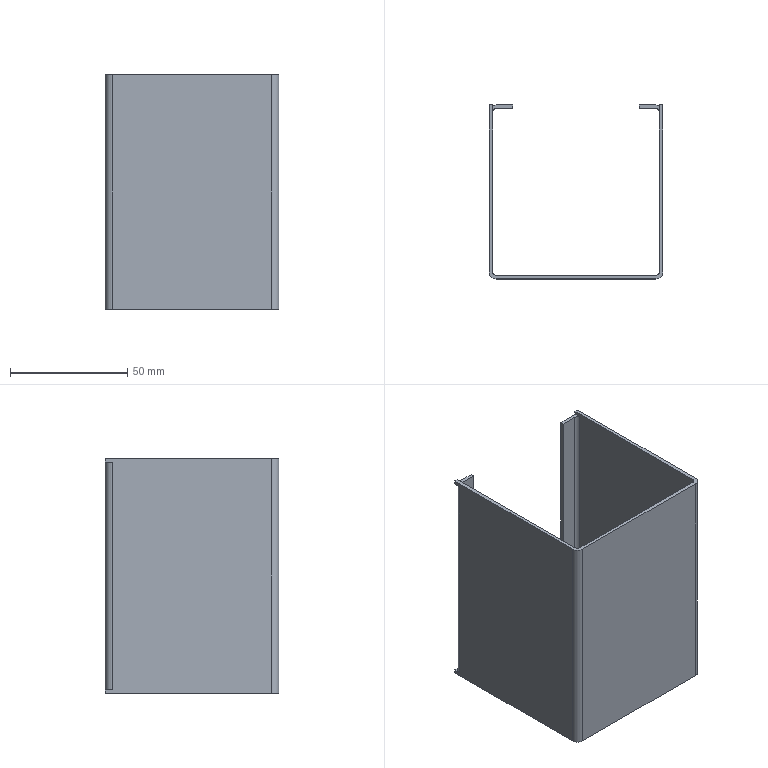Part | NX | features solid 2 | 1 solid | 38 faces | box 74 x 74 x 100 mm | volume 34746 mm3 | plane 30 | cylinder 8 | commonest cylinder face diameters 3 x4 6 x4
STEP:
#1=CARTESIAN_POINT('',(-974.5,-1370.,1296.6));
#2=VERTEX_POINT('',#1);
#3=CARTESIAN_POINT('',(-974.5,-1370.,1393.4));
#4=VERTEX_POINT('',#3);
#5=CARTESIAN_POINT('',(-974.5,-1370.,1296.6));
#6=DIRECTION('',(0.,0.,1.));
#7=VECTOR('',#6,1000.);
#8=LINE('',#5,#7);
#9=EDGE_CURVE('',#2,#4,#8,.T.);
#10=ORIENTED_EDGE('',*,*,#9,.T.);
#11=CARTESIAN_POINT('',(-976.,-1368.5,1393.4));
#12=VERTEX_POINT('',#11);
#13=CARTESIAN_POINT('',(-976.,-1370.,1393.4));
#14=DIRECTION('',(0.,0.,-1.));
#15=DIRECTION('',(1.,0.,0.));
#16=AXIS2_PLACEMENT_3D('',#13,#14,#15);
#17=CIRCLE('',#16,1.5);
#18=EDGE_CURVE('',#12,#4,#17,.T.);
#19=ORIENTED_EDGE('',*,*,#18,.F.);
#20=CARTESIAN_POINT('',(-976.,-1368.5,1296.6));
#21=VERTEX_POINT('',#20);
#22=CARTESIAN_POINT('',(-976.,-1368.5,1393.4));
#23=DIRECTION('',(0.,0.,-1.));
#24=VECTOR('',#23,1000.);
#25=LINE('',#22,#24);
#26=EDGE_CURVE('',#12,#21,#25,.T.);
#27=ORIENTED_EDGE('',*,*,#26,.T.);
#28=CARTESIAN_POINT('',(-976.,-1370.,1296.6));
#29=DIRECTION('',(0.,0.,-1.));
#30=DIRECTION('',(1.,0.,0.));
#31=AXIS2_PLACEMENT_3D('',#28,#29,#30);
#32=CIRCLE('',#31,1.5);
#33=EDGE_CURVE('',#21,#2,#32,.T.);
#34=ORIENTED_EDGE('',*,*,#33,.T.);
#35=EDGE_LOOP('',(#10,#19,#27,#34));
#36=FACE_BOUND('',#35,.T.);
#37=CARTESIAN_POINT('',(-976.,-1370.,1296.6));
#38=DIRECTION('',(0.,0.,1.));
#39=DIRECTION('',(-1.,0.,0.));
#40=AXIS2_PLACEMENT_3D('',#37,#38,#39);
#41=CYLINDRICAL_SURFACE('',#40,1.5);
#42=ADVANCED_FACE('',(#36),#41,.F.);
#43=CARTESIAN_POINT('',(-973.,-1370.,1296.6));
#44=VERTEX_POINT('',#43);
#45=CARTESIAN_POINT('',(-973.,-1370.,1393.4));
#46=VERTEX_POINT('',#45);
#47=CARTESIAN_POINT('',(-973.,-1370.,1296.6));
#48=DIRECTION('',(0.,0.,1.));
#49=VECTOR('',#48,1000.);
#50=LINE('',#47,#49);
#51=EDGE_CURVE('',#44,#46,#50,.T.);
#52=ORIENTED_EDGE('',*,*,#51,.F.);
#53=CARTESIAN_POINT('',(-976.,-1367.,1296.6));
#54=VERTEX_POINT('',#53);
#55=CARTESIAN_POINT('',(-976.,-1370.,1296.6));
#56=DIRECTION('',(0.,0.,-1.));
#57=DIRECTION('',(-1.,0.,0.));
#58=AXIS2_PLACEMENT_3D('',#55,#56,#57);
#59=CIRCLE('',#58,3.);
#60=EDGE_CURVE('',#54,#44,#59,.T.);
#61=ORIENTED_EDGE('',*,*,#60,.F.);
#62=CARTESIAN_POINT('',(-976.,-1367.,1393.4));
#63=VERTEX_POINT('',#62);
#64=CARTESIAN_POINT('',(-976.,-1367.,1393.4));
#65=DIRECTION('',(0.,0.,-1.));
#66=VECTOR('',#65,1000.);
#67=LINE('',#64,#66);
#68=EDGE_CURVE('',#63,#54,#67,.T.);
#69=ORIENTED_EDGE('',*,*,#68,.F.);
#70=CARTESIAN_POINT('',(-976.,-1370.,1393.4));
#71=DIRECTION('',(0.,0.,-1.));
#72=DIRECTION('',(-1.,0.,0.));
#73=AXIS2_PLACEMENT_3D('',#70,#71,#72);
#74=CIRCLE('',#73,3.);
#75=EDGE_CURVE('',#63,#46,#74,.T.);
#76=ORIENTED_EDGE('',*,*,#75,.T.);
#77=EDGE_LOOP('',(#52,#61,#69,#76));
#78=FACE_BOUND('',#77,.T.);
#79=CARTESIAN_POINT('',(-976.,-1370.,1296.6));
#80=DIRECTION('',(0.,0.,1.));
#81=DIRECTION('',(-1.,0.,0.));
#82=AXIS2_PLACEMENT_3D('',#79,#80,#81);
#83=CYLINDRICAL_SURFACE('',#82,3.);
#84=ADVANCED_FACE('',(#78),#83,.T.);
#85=CARTESIAN_POINT('',(-983.,-1368.5,1296.6));
#86=VERTEX_POINT('',#85);
#87=CARTESIAN_POINT('',(-983.,-1368.5,1393.4));
#88=VERTEX_POINT('',#87);
#89=CARTESIAN_POINT('',(-983.,-1368.5,1296.6));
#90=DIRECTION('',(0.,0.,1.));
#91=VECTOR('',#90,1000.);
#92=LINE('',#89,#91);
#93=EDGE_CURVE('',#86,#88,#92,.T.);
#94=ORIENTED_EDGE('',*,*,#93,.T.);
#95=CARTESIAN_POINT('',(-983.,-1367.,1393.4));
#96=VERTEX_POINT('',#95);
#97=CARTESIAN_POINT('',(-983.,-1367.,1393.4));
#98=DIRECTION('',(0.,-1.,0.));
#99=VECTOR('',#98,1000.);
#100=LINE('',#97,#99);
#101=EDGE_CURVE('',#96,#88,#100,.T.);
#102=ORIENTED_EDGE('',*,*,#101,.F.);
#103=CARTESIAN_POINT('',(-983.,-1367.,1296.6));
#104=VERTEX_POINT('',#103);
#105=CARTESIAN_POINT('',(-983.,-1367.,1296.6));
#106=DIRECTION('',(0.,0.,1.));
#107=VECTOR('',#106,1000.);
#108=LINE('',#105,#107);
#109=EDGE_CURVE('',#104,#96,#108,.T.);
#110=ORIENTED_EDGE('',*,*,#109,.F.);
#111=CARTESIAN_POINT('',(-983.,-1367.,1296.6));
#112=DIRECTION('',(0.,-1.,0.));
#113=VECTOR('',#112,1000.);
#114=LINE('',#111,#113);
#115=EDGE_CURVE('',#104,#86,#114,.T.);
#116=ORIENTED_EDGE('',*,*,#115,.T.);
#117=EDGE_LOOP('',(#94,#102,#110,#116));
#118=FACE_BOUND('',#117,.T.);
#119=CARTESIAN_POINT('',(-983.,-1367.,1296.6));
#120=DIRECTION('',(1.,0.,0.));
#121=DIRECTION('',(0.,0.,1.));
#122=AXIS2_PLACEMENT_3D('',#119,#120,#121);
#123=PLANE('',#122);
#124=ADVANCED_FACE('',(#118),#123,.F.);
#125=ORIENTED_EDGE('',*,*,#26,.F.);
#126=CARTESIAN_POINT('',(-983.,-1368.5,1393.4));
#127=DIRECTION('',(1.,0.,0.));
#128=VECTOR('',#127,1000.);
#129=LINE('',#126,#128);
#130=EDGE_CURVE('',#88,#12,#129,.T.);
#131=ORIENTED_EDGE('',*,*,#130,.F.);
#132=ORIENTED_EDGE('',*,*,#93,.F.);
#133=CARTESIAN_POINT('',(-974.351,-1368.5,1296.6));
#134=DIRECTION('',(-1.,0.,0.));
#135=VECTOR('',#134,1000.);
#136=LINE('',#133,#135);
#137=EDGE_CURVE('',#21,#86,#136,.T.);
#138=ORIENTED_EDGE('',*,*,#137,.F.);
#139=EDGE_LOOP('',(#125,#131,#132,#138));
#140=FACE_BOUND('',#139,.T.);
#141=CARTESIAN_POINT('',(-1010.,-1368.5,1345.));
#142=DIRECTION('',(0.,1.,0.));
#143=DIRECTION('',(1.,0.,0.));
#144=AXIS2_PLACEMENT_3D('',#141,#142,#143);
#145=PLANE('',#144);
#146=ADVANCED_FACE('',(#140),#145,.F.);
#147=CARTESIAN_POINT('',(-983.,-1367.,1393.4));
#148=DIRECTION('',(1.,0.,0.));
#149=VECTOR('',#148,1000.);
#150=LINE('',#147,#149);
#151=EDGE_CURVE('',#96,#63,#150,.T.);
#152=ORIENTED_EDGE('',*,*,#151,.T.);
#153=ORIENTED_EDGE('',*,*,#68,.T.);
#154=CARTESIAN_POINT('',(-974.351,-1367.,1296.6));
#155=DIRECTION('',(-1.,0.,0.));
#156=VECTOR('',#155,1000.);
#157=LINE('',#154,#156);
#158=EDGE_CURVE('',#54,#104,#157,.T.);
#159=ORIENTED_EDGE('',*,*,#158,.T.);
#160=ORIENTED_EDGE('',*,*,#109,.T.);
#161=EDGE_LOOP('',(#152,#153,#159,#160));
#162=FACE_BOUND('',#161,.T.);
#163=CARTESIAN_POINT('',(-1010.,-1367.,1345.));
#164=DIRECTION('',(0.,1.,0.));
#165=DIRECTION('',(1.,0.,0.));
#166=AXIS2_PLACEMENT_3D('',#163,#164,#165);
#167=PLANE('',#166);
#168=ADVANCED_FACE('',(#162),#167,.T.);
#169=CARTESIAN_POINT('',(-974.5,-1370.1,1393.5));
#170=VERTEX_POINT('',#169);
#171=CARTESIAN_POINT('',(-973.,-1370.1,1393.5));
#172=VERTEX_POINT('',#171);
#173=CARTESIAN_POINT('',(-973.,-1370.1,1393.5));
#174=DIRECTION('',(1.,0.,0.));
#175=VECTOR('',#174,1000.);
#176=LINE('',#173,#175);
#177=EDGE_CURVE('',#170,#172,#176,.T.);
#178=ORIENTED_EDGE('',*,*,#177,.T.);
#179=CARTESIAN_POINT('',(-973.,-1370.1,1393.4));
#180=VERTEX_POINT('',#179);
#181=CARTESIAN_POINT('',(-973.,-1370.1,1393.5));
#182=DIRECTION('',(0.,0.,1.));
#183=VECTOR('',#182,1000.);
#184=LINE('',#181,#183);
#185=EDGE_CURVE('',#180,#172,#184,.T.);
#186=ORIENTED_EDGE('',*,*,#185,.F.);
#187=CARTESIAN_POINT('',(-974.5,-1370.1,1393.4));
#188=VERTEX_POINT('',#187);
#189=CARTESIAN_POINT('',(-973.,-1370.1,1393.4));
#190=DIRECTION('',(1.,0.,0.));
#191=VECTOR('',#190,1000.);
#192=LINE('',#189,#191);
#193=EDGE_CURVE('',#188,#180,#192,.T.);
#194=ORIENTED_EDGE('',*,*,#193,.F.);
#195=CARTESIAN_POINT('',(-974.5,-1370.1,1393.4));
#196=DIRECTION('',(0.,0.,1.));
#197=VECTOR('',#196,1000.);
#198=LINE('',#195,#197);
#199=EDGE_CURVE('',#188,#170,#198,.T.);
#200=ORIENTED_EDGE('',*,*,#199,.T.);
#201=EDGE_LOOP('',(#178,#186,#194,#200));
#202=FACE_BOUND('',#201,.T.);
#203=CARTESIAN_POINT('',(-973.,-1370.1,1393.5));
#204=DIRECTION('',(0.,-1.,0.));
#205=DIRECTION('',(0.,0.,-1.));
#206=AXIS2_PLACEMENT_3D('',#203,#204,#205);
#207=PLANE('',#206);
#208=ADVANCED_FACE('',(#202),#207,.F.);
#209=CARTESIAN_POINT('',(-974.5,-1367.,1393.5));
#210=VERTEX_POINT('',#209);
#211=CARTESIAN_POINT('',(-973.,-1367.,1393.5));
#212=VERTEX_POINT('',#211);
#213=CARTESIAN_POINT('',(-973.,-1367.,1393.5));
#214=DIRECTION('',(1.,0.,0.));
#215=VECTOR('',#214,1000.);
#216=LINE('',#213,#215);
#217=EDGE_CURVE('',#210,#212,#216,.T.);
#218=ORIENTED_EDGE('',*,*,#217,.T.);
#219=CARTESIAN_POINT('',(-973.,-1367.,1393.5));
#220=DIRECTION('',(0.,1.,0.));
#221=VECTOR('',#220,1000.);
#222=LINE('',#219,#221);
#223=EDGE_CURVE('',#172,#212,#222,.T.);
#224=ORIENTED_EDGE('',*,*,#223,.F.);
#225=ORIENTED_EDGE('',*,*,#177,.F.);
#226=CARTESIAN_POINT('',(-974.5,-1370.1,1393.5));
#227=DIRECTION('',(0.,1.,0.));
#228=VECTOR('',#227,1000.);
#229=LINE('',#226,#228);
#230=EDGE_CURVE('',#170,#210,#229,.T.);
#231=ORIENTED_EDGE('',*,*,#230,.T.);
#232=EDGE_LOOP('',(#218,#224,#225,#231));
#233=FACE_BOUND('',#232,.T.);
#234=CARTESIAN_POINT('',(-973.,-1367.,1393.5));
#235=DIRECTION('',(0.,0.,1.));
#236=DIRECTION('',(0.,-1.,0.));
#237=AXIS2_PLACEMENT_3D('',#234,#235,#236);
#238=PLANE('',#237);
#239=ADVANCED_FACE('',(#233),#238,.F.);
#240=CARTESIAN_POINT('',(-974.5,-1370.1,1296.6));
#241=VERTEX_POINT('',#240);
#242=CARTESIAN_POINT('',(-974.5,-1370.1,1296.5));
#243=VERTEX_POINT('',#242);
#244=CARTESIAN_POINT('',(-974.5,-1370.1,1296.6));
#245=DIRECTION('',(0.,0.,-1.));
#246=VECTOR('',#245,1000.);
#247=LINE('',#244,#246);
#248=EDGE_CURVE('',#241,#243,#247,.T.);
#249=ORIENTED_EDGE('',*,*,#248,.F.);
#250=CARTESIAN_POINT('',(-973.,-1370.1,1296.6));
#251=VERTEX_POINT('',#250);
#252=CARTESIAN_POINT('',(-973.,-1370.1,1296.6));
#253=DIRECTION('',(1.,0.,0.));
#254=VECTOR('',#253,1000.);
#255=LINE('',#252,#254);
#256=EDGE_CURVE('',#241,#251,#255,.T.);
#257=ORIENTED_EDGE('',*,*,#256,.T.);
#258=CARTESIAN_POINT('',(-973.,-1370.1,1296.5));
#259=VERTEX_POINT('',#258);
#260=CARTESIAN_POINT('',(-973.,-1370.1,1296.5));
#261=DIRECTION('',(0.,0.,-1.));
#262=VECTOR('',#261,1000.);
#263=LINE('',#260,#262);
#264=EDGE_CURVE('',#251,#259,#263,.T.);
#265=ORIENTED_EDGE('',*,*,#264,.T.);
#266=CARTESIAN_POINT('',(-973.,-1370.1,1296.5));
#267=DIRECTION('',(1.,0.,0.));
#268=VECTOR('',#267,1000.);
#269=LINE('',#266,#268);
#270=EDGE_CURVE('',#243,#259,#269,.T.);
#271=ORIENTED_EDGE('',*,*,#270,.F.);
#272=EDGE_LOOP('',(#249,#257,#265,#271));
#273=FACE_BOUND('',#272,.T.);
#274=CARTESIAN_POINT('',(-973.,-1370.1,1296.5));
#275=DIRECTION('',(0.,-1.,0.));
#276=DIRECTION('',(0.,0.,-1.));
#277=AXIS2_PLACEMENT_3D('',#274,#275,#276);
#278=PLANE('',#277);
#279=ADVANCED_FACE('',(#273),#278,.F.);
#280=ORIENTED_EDGE('',*,*,#270,.T.);
#281=CARTESIAN_POINT('',(-973.,-1367.,1296.5));
#282=VERTEX_POINT('',#281);
#283=CARTESIAN_POINT('',(-973.,-1367.,1296.5));
#284=DIRECTION('',(0.,1.,0.));
#285=VECTOR('',#284,1000.);
#286=LINE('',#283,#285);
#287=EDGE_CURVE('',#259,#282,#286,.T.);
#288=ORIENTED_EDGE('',*,*,#287,.T.);
#289=CARTESIAN_POINT('',(-974.5,-1367.,1296.5));
#290=VERTEX_POINT('',#289);
#291=CARTESIAN_POINT('',(-973.,-1367.,1296.5));
#292=DIRECTION('',(1.,0.,0.));
#293=VECTOR('',#292,1000.);
#294=LINE('',#291,#293);
#295=EDGE_CURVE('',#290,#282,#294,.T.);
#296=ORIENTED_EDGE('',*,*,#295,.F.);
#297=CARTESIAN_POINT('',(-974.5,-1370.1,1296.5));
#298=DIRECTION('',(0.,1.,0.));
#299=VECTOR('',#298,1000.);
#300=LINE('',#297,#299);
#301=EDGE_CURVE('',#243,#290,#300,.T.);
#302=ORIENTED_EDGE('',*,*,#301,.F.);
#303=EDGE_LOOP('',(#280,#288,#296,#302));
#304=FACE_BOUND('',#303,.T.);
#305=CARTESIAN_POINT('',(-973.,-1367.,1296.5));
#306=DIRECTION('',(0.,0.,-1.));
#307=DIRECTION('',(0.,-1.,0.));
#308=AXIS2_PLACEMENT_3D('',#305,#306,#307);
#309=PLANE('',#308);
#310=ADVANCED_FACE('',(#304),#309,.F.);
#311=CARTESIAN_POINT('',(-1045.5,-1370.,1393.4));
#312=VERTEX_POINT('',#311);
#313=CARTESIAN_POINT('',(-1045.5,-1370.,1296.6));
#314=VERTEX_POINT('',#313);
#315=CARTESIAN_POINT('',(-1045.5,-1370.,1393.4));
#316=DIRECTION('',(0.,0.,-1.));
#317=VECTOR('',#316,1000.);
#318=LINE('',#315,#317);
#319=EDGE_CURVE('',#312,#314,#318,.T.);
#320=ORIENTED_EDGE('',*,*,#319,.T.);
#321=CARTESIAN_POINT('',(-1044.,-1368.5,1296.6));
#322=VERTEX_POINT('',#321);
#323=CARTESIAN_POINT('',(-1044.,-1370.,1296.6));
#324=DIRECTION('',(0.,0.,1.));
#325=DIRECTION('',(-1.,0.,0.));
#326=AXIS2_PLACEMENT_3D('',#323,#324,#325);
#327=CIRCLE('',#326,1.5);
#328=EDGE_CURVE('',#322,#314,#327,.T.);
#329=ORIENTED_EDGE('',*,*,#328,.F.);
#330=CARTESIAN_POINT('',(-1044.,-1368.5,1393.4));
#331=VERTEX_POINT('',#330);
#332=CARTESIAN_POINT('',(-1044.,-1368.5,1296.6));
#333=DIRECTION('',(0.,0.,1.));
#334=VECTOR('',#333,1000.);
#335=LINE('',#332,#334);
#336=EDGE_CURVE('',#322,#331,#335,.T.);
#337=ORIENTED_EDGE('',*,*,#336,.T.);
#338=CARTESIAN_POINT('',(-1044.,-1370.,1393.4));
#339=DIRECTION('',(0.,0.,1.));
#340=DIRECTION('',(-1.,0.,0.));
#341=AXIS2_PLACEMENT_3D('',#338,#339,#340);
#342=CIRCLE('',#341,1.5);
#343=EDGE_CURVE('',#331,#312,#342,.T.);
#344=ORIENTED_EDGE('',*,*,#343,.T.);
#345=EDGE_LOOP('',(#320,#329,#337,#344));
#346=FACE_BOUND('',#345,.T.);
#347=CARTESIAN_POINT('',(-1044.,-1370.,1393.4));
#348=DIRECTION('',(0.,0.,-1.));
#349=DIRECTION('',(1.,0.,0.));
#350=AXIS2_PLACEMENT_3D('',#347,#348,#349);
#351=CYLINDRICAL_SURFACE('',#350,1.5);
#352=ADVANCED_FACE('',(#346),#351,.F.);
#353=CARTESIAN_POINT('',(-1047.,-1370.,1393.4));
#354=VERTEX_POINT('',#353);
#355=CARTESIAN_POINT('',(-1047.,-1370.,1296.6));
#356=VERTEX_POINT('',#355);
#357=CARTESIAN_POINT('',(-1047.,-1370.,1393.4));
#358=DIRECTION('',(0.,0.,-1.));
#359=VECTOR('',#358,1000.);
#360=LINE('',#357,#359);
#361=EDGE_CURVE('',#354,#356,#360,.T.);
#362=ORIENTED_EDGE('',*,*,#361,.F.);
#363=CARTESIAN_POINT('',(-1044.,-1367.,1393.4));
#364=VERTEX_POINT('',#363);
#365=CARTESIAN_POINT('',(-1044.,-1370.,1393.4));
#366=DIRECTION('',(0.,0.,1.));
#367=DIRECTION('',(1.,0.,0.));
#368=AXIS2_PLACEMENT_3D('',#365,#366,#367);
#369=CIRCLE('',#368,3.);
#370=EDGE_CURVE('',#364,#354,#369,.T.);
#371=ORIENTED_EDGE('',*,*,#370,.F.);
#372=CARTESIAN_POINT('',(-1044.,-1367.,1296.6));
#373=VERTEX_POINT('',#372);
#374=CARTESIAN_POINT('',(-1044.,-1367.,1296.6));
#375=DIRECTION('',(0.,0.,1.));
#376=VECTOR('',#375,1000.);
#377=LINE('',#374,#376);
#378=EDGE_CURVE('',#373,#364,#377,.T.);
#379=ORIENTED_EDGE('',*,*,#378,.F.);
#380=CARTESIAN_POINT('',(-1044.,-1370.,1296.6));
#381=DIRECTION('',(0.,0.,1.));
#382=DIRECTION('',(1.,0.,0.));
#383=AXIS2_PLACEMENT_3D('',#380,#381,#382);
#384=CIRCLE('',#383,3.);
#385=EDGE_CURVE('',#373,#356,#384,.T.);
#386=ORIENTED_EDGE('',*,*,#385,.T.);
#387=EDGE_LOOP('',(#362,#371,#379,#386));
#388=FACE_BOUND('',#387,.T.);
#389=CARTESIAN_POINT('',(-1044.,-1370.,1393.4));
#390=DIRECTION('',(0.,0.,-1.));
#391=DIRECTION('',(1.,0.,0.));
#392=AXIS2_PLACEMENT_3D('',#389,#390,#391);
#393=CYLINDRICAL_SURFACE('',#392,3.);
#394=ADVANCED_FACE('',(#388),#393,.T.);
#395=CARTESIAN_POINT('',(-1037.,-1368.5,1393.4));
#396=VERTEX_POINT('',#395);
#397=CARTESIAN_POINT('',(-1037.,-1368.5,1296.6));
#398=VERTEX_POINT('',#397);
#399=CARTESIAN_POINT('',(-1037.,-1368.5,1393.4));
#400=DIRECTION('',(0.,0.,-1.));
#401=VECTOR('',#400,1000.);
#402=LINE('',#399,#401);
#403=EDGE_CURVE('',#396,#398,#402,.T.);
#404=ORIENTED_EDGE('',*,*,#403,.T.);
#405=CARTESIAN_POINT('',(-1037.,-1367.,1296.6));
#406=VERTEX_POINT('',#405);
#407=CARTESIAN_POINT('',(-1037.,-1367.,1296.6));
#408=DIRECTION('',(0.,-1.,0.));
#409=VECTOR('',#408,1000.);
#410=LINE('',#407,#409);
#411=EDGE_CURVE('',#406,#398,#410,.T.);
#412=ORIENTED_EDGE('',*,*,#411,.F.);
#413=CARTESIAN_POINT('',(-1037.,-1367.,1393.4));
#414=VERTEX_POINT('',#413);
#415=CARTESIAN_POINT('',(-1037.,-1367.,1393.4));
#416=DIRECTION('',(0.,0.,-1.));
#417=VECTOR('',#416,1000.);
#418=LINE('',#415,#417);
#419=EDGE_CURVE('',#414,#406,#418,.T.);
#420=ORIENTED_EDGE('',*,*,#419,.F.);
#421=CARTESIAN_POINT('',(-1037.,-1367.,1393.4));
#422=DIRECTION('',(0.,-1.,0.));
#423=VECTOR('',#422,1000.);
#424=LINE('',#421,#423);
#425=EDGE_CURVE('',#414,#396,#424,.T.);
#426=ORIENTED_EDGE('',*,*,#425,.T.);
#427=EDGE_LOOP('',(#404,#412,#420,#426));
#428=FACE_BOUND('',#427,.T.);
#429=CARTESIAN_POINT('',(-1037.,-1367.,1393.4));
#430=DIRECTION('',(-1.,0.,0.));
#431=DIRECTION('',(0.,1.,0.));
#432=AXIS2_PLACEMENT_3D('',#429,#430,#431);
#433=PLANE('',#432);
#434=ADVANCED_FACE('',(#428),#433,.F.);
#435=ORIENTED_EDGE('',*,*,#336,.F.);
#436=CARTESIAN_POINT('',(-1045.649,-1368.5,1296.6));
#437=DIRECTION('',(-1.,0.,0.));
#438=VECTOR('',#437,1000.);
#439=LINE('',#436,#438);
#440=EDGE_CURVE('',#398,#322,#439,.T.);
#441=ORIENTED_EDGE('',*,*,#440,.F.);
#442=ORIENTED_EDGE('',*,*,#403,.F.);
#443=CARTESIAN_POINT('',(-1045.649,-1368.5,1393.4));
#444=DIRECTION('',(1.,0.,0.));
#445=VECTOR('',#444,1000.);
#446=LINE('',#443,#445);
#447=EDGE_CURVE('',#331,#396,#446,.T.);
#448=ORIENTED_EDGE('',*,*,#447,.F.);
#449=EDGE_LOOP('',(#435,#441,#442,#448));
#450=FACE_BOUND('',#449,.T.);
#451=CARTESIAN_POINT('',(-1010.,-1368.5,1345.));
#452=DIRECTION('',(0.,1.,0.));
#453=DIRECTION('',(1.,0.,0.));
#454=AXIS2_PLACEMENT_3D('',#451,#452,#453);
#455=PLANE('',#454);
#456=ADVANCED_FACE('',(#450),#455,.F.);
#457=CARTESIAN_POINT('',(-1045.649,-1367.,1296.6));
#458=DIRECTION('',(-1.,0.,0.));
#459=VECTOR('',#458,1000.);
#460=LINE('',#457,#459);
#461=EDGE_CURVE('',#406,#373,#460,.T.);
#462=ORIENTED_EDGE('',*,*,#461,.T.);
#463=ORIENTED_EDGE('',*,*,#378,.T.);
#464=CARTESIAN_POINT('',(-1045.649,-1367.,1393.4));
#465=DIRECTION('',(1.,0.,0.));
#466=VECTOR('',#465,1000.);
#467=LINE('',#464,#466);
#468=EDGE_CURVE('',#364,#414,#467,.T.);
#469=ORIENTED_EDGE('',*,*,#468,.T.);
#470=ORIENTED_EDGE('',*,*,#419,.T.);
#471=EDGE_LOOP('',(#462,#463,#469,#470));
#472=FACE_BOUND('',#471,.T.);
#473=CARTESIAN_POINT('',(-1010.,-1367.,1345.));
#474=DIRECTION('',(0.,1.,0.));
#475=DIRECTION('',(1.,0.,0.));
#476=AXIS2_PLACEMENT_3D('',#473,#474,#475);
#477=PLANE('',#476);
#478=ADVANCED_FACE('',(#472),#477,.T.);
#479=CARTESIAN_POINT('',(-1045.5,-1370.1,1296.5));
#480=VERTEX_POINT('',#479);
#481=CARTESIAN_POINT('',(-1047.,-1370.1,1296.5));
#482=VERTEX_POINT('',#481);
#483=CARTESIAN_POINT('',(-1047.,-1370.1,1296.5));
#484=DIRECTION('',(-1.,0.,0.));
#485=VECTOR('',#484,1000.);
#486=LINE('',#483,#485);
#487=EDGE_CURVE('',#480,#482,#486,.T.);
#488=ORIENTED_EDGE('',*,*,#487,.T.);
#489=CARTESIAN_POINT('',(-1047.,-1370.1,1296.6));
#490=VERTEX_POINT('',#489);
#491=CARTESIAN_POINT('',(-1047.,-1370.1,1296.5));
#492=DIRECTION('',(0.,0.,-1.));
#493=VECTOR('',#492,1000.);
#494=LINE('',#491,#493);
#495=EDGE_CURVE('',#490,#482,#494,.T.);
#496=ORIENTED_EDGE('',*,*,#495,.F.);
#497=CARTESIAN_POINT('',(-1045.5,-1370.1,1296.6));
#498=VERTEX_POINT('',#497);
#499=CARTESIAN_POINT('',(-1047.,-1370.1,1296.6));
#500=DIRECTION('',(-1.,0.,0.));
#501=VECTOR('',#500,1000.);
#502=LINE('',#499,#501);
#503=EDGE_CURVE('',#498,#490,#502,.T.);
#504=ORIENTED_EDGE('',*,*,#503,.F.);
#505=CARTESIAN_POINT('',(-1045.5,-1370.1,1296.6));
#506=DIRECTION('',(0.,0.,-1.));
#507=VECTOR('',#506,1000.);
#508=LINE('',#505,#507);
#509=EDGE_CURVE('',#498,#480,#508,.T.);
#510=ORIENTED_EDGE('',*,*,#509,.T.);
#511=EDGE_LOOP('',(#488,#496,#504,#510));
#512=FACE_BOUND('',#511,.T.);
#513=CARTESIAN_POINT('',(-1047.,-1370.1,1296.5));
#514=DIRECTION('',(0.,-1.,0.));
#515=DIRECTION('',(0.,0.,-1.));
#516=AXIS2_PLACEMENT_3D('',#513,#514,#515);
#517=PLANE('',#516);
#518=ADVANCED_FACE('',(#512),#517,.F.);
#519=CARTESIAN_POINT('',(-1045.5,-1367.,1296.5));
#520=VERTEX_POINT('',#519);
#521=CARTESIAN_POINT('',(-1047.,-1367.,1296.5));
#522=VERTEX_POINT('',#521);
#523=CARTESIAN_POINT('',(-1047.,-1367.,1296.5));
#524=DIRECTION('',(-1.,0.,0.));
#525=VECTOR('',#524,1000.);
#526=LINE('',#523,#525);
#527=EDGE_CURVE('',#520,#522,#526,.T.);
#528=ORIENTED_EDGE('',*,*,#527,.T.);
#529=CARTESIAN_POINT('',(-1047.,-1367.,1296.5));
#530=DIRECTION('',(0.,1.,0.));
#531=VECTOR('',#530,1000.);
#532=LINE('',#529,#531);
#533=EDGE_CURVE('',#482,#522,#532,.T.);
#534=ORIENTED_EDGE('',*,*,#533,.F.);
#535=ORIENTED_EDGE('',*,*,#487,.F.);
#536=CARTESIAN_POINT('',(-1045.5,-1370.1,1296.5));
#537=DIRECTION('',(0.,1.,0.));
#538=VECTOR('',#537,1000.);
#539=LINE('',#536,#538);
#540=EDGE_CURVE('',#480,#520,#539,.T.);
#541=ORIENTED_EDGE('',*,*,#540,.T.);
#542=EDGE_LOOP('',(#528,#534,#535,#541));
#543=FACE_BOUND('',#542,.T.);
#544=CARTESIAN_POINT('',(-1047.,-1367.,1296.5));
#545=DIRECTION('',(0.,0.,-1.));
#546=DIRECTION('',(0.,-1.,0.));
#547=AXIS2_PLACEMENT_3D('',#544,#545,#546);
#548=PLANE('',#547);
#549=ADVANCED_FACE('',(#543),#548,.F.);
#550=CARTESIAN_POINT('',(-1045.5,-1370.1,1393.4));
#551=VERTEX_POINT('',#550);
#552=CARTESIAN_POINT('',(-1045.5,-1370.1,1393.5));
#553=VERTEX_POINT('',#552);
#554=CARTESIAN_POINT('',(-1045.5,-1370.1,1393.4));
#555=DIRECTION('',(0.,0.,1.));
#556=VECTOR('',#555,1000.);
#557=LINE('',#554,#556);
#558=EDGE_CURVE('',#551,#553,#557,.T.);
#559=ORIENTED_EDGE('',*,*,#558,.F.);
#560=CARTESIAN_POINT('',(-1047.,-1370.1,1393.4));
#561=VERTEX_POINT('',#560);
#562=CARTESIAN_POINT('',(-1047.,-1370.1,1393.4));
#563=DIRECTION('',(-1.,0.,0.));
#564=VECTOR('',#563,1000.);
#565=LINE('',#562,#564);
#566=EDGE_CURVE('',#551,#561,#565,.T.);
#567=ORIENTED_EDGE('',*,*,#566,.T.);
#568=CARTESIAN_POINT('',(-1047.,-1370.1,1393.5));
#569=VERTEX_POINT('',#568);
#570=CARTESIAN_POINT('',(-1047.,-1370.1,1393.5));
#571=DIRECTION('',(0.,0.,1.));
#572=VECTOR('',#571,1000.);
#573=LINE('',#570,#572);
#574=EDGE_CURVE('',#561,#569,#573,.T.);
#575=ORIENTED_EDGE('',*,*,#574,.T.);
#576=CARTESIAN_POINT('',(-1047.,-1370.1,1393.5));
#577=DIRECTION('',(-1.,0.,0.));
#578=VECTOR('',#577,1000.);
#579=LINE('',#576,#578);
#580=EDGE_CURVE('',#553,#569,#579,.T.);
#581=ORIENTED_EDGE('',*,*,#580,.F.);
#582=EDGE_LOOP('',(#559,#567,#575,#581));
#583=FACE_BOUND('',#582,.T.);
#584=CARTESIAN_POINT('',(-1047.,-1370.1,1393.5));
#585=DIRECTION('',(0.,-1.,0.));
#586=DIRECTION('',(0.,0.,-1.));
#587=AXIS2_PLACEMENT_3D('',#584,#585,#586);
#588=PLANE('',#587);
#589=ADVANCED_FACE('',(#583),#588,.F.);
#590=ORIENTED_EDGE('',*,*,#580,.T.);
#591=CARTESIAN_POINT('',(-1047.,-1367.,1393.5));
#592=VERTEX_POINT('',#591);
#593=CARTESIAN_POINT('',(-1047.,-1367.,1393.5));
#594=DIRECTION('',(0.,1.,0.));
#595=VECTOR('',#594,1000.);
#596=LINE('',#593,#595);
#597=EDGE_CURVE('',#569,#592,#596,.T.);
#598=ORIENTED_EDGE('',*,*,#597,.T.);
#599=CARTESIAN_POINT('',(-1045.5,-1367.,1393.5));
#600=VERTEX_POINT('',#599);
#601=CARTESIAN_POINT('',(-1047.,-1367.,1393.5));
#602=DIRECTION('',(-1.,0.,0.));
#603=VECTOR('',#602,1000.);
#604=LINE('',#601,#603);
#605=EDGE_CURVE('',#600,#592,#604,.T.);
#606=ORIENTED_EDGE('',*,*,#605,.F.);
#607=CARTESIAN_POINT('',(-1045.5,-1370.1,1393.5));
#608=DIRECTION('',(0.,1.,0.));
#609=VECTOR('',#608,1000.);
#610=LINE('',#607,#609);
#611=EDGE_CURVE('',#553,#600,#610,.T.);
#612=ORIENTED_EDGE('',*,*,#611,.F.);
#613=EDGE_LOOP('',(#590,#598,#606,#612));
#614=FACE_BOUND('',#613,.T.);
#615=CARTESIAN_POINT('',(-1047.,-1367.,1393.5));
#616=DIRECTION('',(0.,0.,1.));
#617=DIRECTION('',(1.,0.,0.));
#618=AXIS2_PLACEMENT_3D('',#615,#616,#617);
#619=PLANE('',#618);
#620=ADVANCED_FACE('',(#614),#619,.F.);
#621=ORIENTED_EDGE('',*,*,#9,.F.);
#622=CARTESIAN_POINT('',(-974.5,-1370.1,1296.6));
#623=DIRECTION('',(0.,-1.,0.));
#624=VECTOR('',#623,1000.);
#625=LINE('',#622,#624);
#626=EDGE_CURVE('',#2,#241,#625,.T.);
#627=ORIENTED_EDGE('',*,*,#626,.T.);
#628=ORIENTED_EDGE('',*,*,#248,.T.);
#629=ORIENTED_EDGE('',*,*,#301,.T.);
#630=CARTESIAN_POINT('',(-974.5,-1367.,1295.));
#631=VERTEX_POINT('',#630);
#632=CARTESIAN_POINT('',(-974.5,-1367.,1295.));
#633=DIRECTION('',(0.,0.,1.));
#634=VECTOR('',#633,1000.);
#635=LINE('',#632,#634);
#636=EDGE_CURVE('',#631,#290,#635,.T.);
#637=ORIENTED_EDGE('',*,*,#636,.F.);
#638=CARTESIAN_POINT('',(-974.5,-1438.,1295.));
#639=VERTEX_POINT('',#638);
#640=CARTESIAN_POINT('',(-974.5,-1441.,1295.));
#641=DIRECTION('',(0.,1.,0.));
#642=VECTOR('',#641,1000.);
#643=LINE('',#640,#642);
#644=EDGE_CURVE('',#639,#631,#643,.T.);
#645=ORIENTED_EDGE('',*,*,#644,.F.);
#646=CARTESIAN_POINT('',(-974.5,-1438.,1395.));
#647=VERTEX_POINT('',#646);
#648=CARTESIAN_POINT('',(-974.5,-1438.,1295.));
#649=DIRECTION('',(0.,0.,1.));
#650=VECTOR('',#649,1000.);
#651=LINE('',#648,#650);
#652=EDGE_CURVE('',#639,#647,#651,.T.);
#653=ORIENTED_EDGE('',*,*,#652,.T.);
#654=CARTESIAN_POINT('',(-974.5,-1367.,1395.));
#655=VERTEX_POINT('',#654);
#656=CARTESIAN_POINT('',(-974.5,-1441.,1395.));
#657=DIRECTION('',(0.,1.,0.));
#658=VECTOR('',#657,1000.);
#659=LINE('',#656,#658);
#660=EDGE_CURVE('',#647,#655,#659,.T.);
#661=ORIENTED_EDGE('',*,*,#660,.T.);
#662=CARTESIAN_POINT('',(-974.5,-1367.,1295.));
#663=DIRECTION('',(0.,0.,1.));
#664=VECTOR('',#663,1000.);
#665=LINE('',#662,#664);
#666=EDGE_CURVE('',#210,#655,#665,.T.);
#667=ORIENTED_EDGE('',*,*,#666,.F.);
#668=ORIENTED_EDGE('',*,*,#230,.F.);
#669=ORIENTED_EDGE('',*,*,#199,.F.);
#670=CARTESIAN_POINT('',(-974.5,-1370.1,1393.4));
#671=DIRECTION('',(0.,-1.,0.));
#672=VECTOR('',#671,1000.);
#673=LINE('',#670,#672);
#674=EDGE_CURVE('',#4,#188,#673,.T.);
#675=ORIENTED_EDGE('',*,*,#674,.F.);
#676=EDGE_LOOP('',(#621,#627,#628,#629,#637,#645,#653,#661,#667,#668,#669,#675));
#677=FACE_BOUND('',#676,.T.);
#678=CARTESIAN_POINT('',(-974.5,-1441.,1295.));
#679=DIRECTION('',(1.,0.,0.));
#680=DIRECTION('',(0.,1.,0.));
#681=AXIS2_PLACEMENT_3D('',#678,#679,#680);
#682=PLANE('',#681);
#683=ADVANCED_FACE('',(#677),#682,.F.);
#684=CARTESIAN_POINT('',(-976.,-1439.5,1395.));
#685=VERTEX_POINT('',#684);
#686=CARTESIAN_POINT('',(-976.,-1438.,1395.));
#687=DIRECTION('',(0.,0.,1.));
#688=DIRECTION('',(1.,0.,0.));
#689=AXIS2_PLACEMENT_3D('',#686,#687,#688);
#690=CIRCLE('',#689,1.5);
#691=EDGE_CURVE('',#685,#647,#690,.T.);
#692=ORIENTED_EDGE('',*,*,#691,.T.);
#693=ORIENTED_EDGE('',*,*,#652,.F.);
#694=CARTESIAN_POINT('',(-976.,-1439.5,1295.));
#695=VERTEX_POINT('',#694);
#696=CARTESIAN_POINT('',(-976.,-1438.,1295.));
#697=DIRECTION('',(0.,0.,1.));
#698=DIRECTION('',(1.,0.,0.));
#699=AXIS2_PLACEMENT_3D('',#696,#697,#698);
#700=CIRCLE('',#699,1.5);
#701=EDGE_CURVE('',#695,#639,#700,.T.);
#702=ORIENTED_EDGE('',*,*,#701,.F.);
#703=CARTESIAN_POINT('',(-976.,-1439.5,1295.));
#704=DIRECTION('',(0.,0.,1.));
#705=VECTOR('',#704,1000.);
#706=LINE('',#703,#705);
#707=EDGE_CURVE('',#695,#685,#706,.T.);
#708=ORIENTED_EDGE('',*,*,#707,.T.);
#709=EDGE_LOOP('',(#692,#693,#702,#708));
#710=FACE_BOUND('',#709,.T.);
#711=CARTESIAN_POINT('',(-976.,-1438.,1295.));
#712=DIRECTION('',(0.,0.,1.));
#713=DIRECTION('',(1.,0.,0.));
#714=AXIS2_PLACEMENT_3D('',#711,#712,#713);
#715=CYLINDRICAL_SURFACE('',#714,1.5);
#716=ADVANCED_FACE('',(#710),#715,.F.);
#717=CARTESIAN_POINT('',(-1044.,-1439.5,1395.));
#718=VERTEX_POINT('',#717);
#719=CARTESIAN_POINT('',(-1047.,-1439.5,1395.));
#720=DIRECTION('',(1.,0.,0.));
#721=VECTOR('',#720,1000.);
#722=LINE('',#719,#721);
#723=EDGE_CURVE('',#718,#685,#722,.T.);
#724=ORIENTED_EDGE('',*,*,#723,.T.);
#725=ORIENTED_EDGE('',*,*,#707,.F.);
#726=CARTESIAN_POINT('',(-1044.,-1439.5,1295.));
#727=VERTEX_POINT('',#726);
#728=CARTESIAN_POINT('',(-1047.,-1439.5,1295.));
#729=DIRECTION('',(1.,0.,0.));
#730=VECTOR('',#729,1000.);
#731=LINE('',#728,#730);
#732=EDGE_CURVE('',#727,#695,#731,.T.);
#733=ORIENTED_EDGE('',*,*,#732,.F.);
#734=CARTESIAN_POINT('',(-1044.,-1439.5,1295.));
#735=DIRECTION('',(0.,0.,1.));
#736=VECTOR('',#735,1000.);
#737=LINE('',#734,#736);
#738=EDGE_CURVE('',#727,#718,#737,.T.);
#739=ORIENTED_EDGE('',*,*,#738,.T.);
#740=EDGE_LOOP('',(#724,#725,#733,#739));
#741=FACE_BOUND('',#740,.T.);
#742=CARTESIAN_POINT('',(-1047.,-1439.5,1295.));
#743=DIRECTION('',(0.,-1.,0.));
#744=DIRECTION('',(-1.,0.,0.));
#745=AXIS2_PLACEMENT_3D('',#742,#743,#744);
#746=PLANE('',#745);
#747=ADVANCED_FACE('',(#741),#746,.F.);
#748=CARTESIAN_POINT('',(-1045.5,-1438.,1395.));
#749=VERTEX_POINT('',#748);
#750=CARTESIAN_POINT('',(-1044.,-1438.,1395.));
#751=DIRECTION('',(0.,0.,1.));
#752=DIRECTION('',(1.,0.,0.));
#753=AXIS2_PLACEMENT_3D('',#750,#751,#752);
#754=CIRCLE('',#753,1.5);
#755=EDGE_CURVE('',#749,#718,#754,.T.);
#756=ORIENTED_EDGE('',*,*,#755,.T.);
#757=ORIENTED_EDGE('',*,*,#738,.F.);
#758=CARTESIAN_POINT('',(-1045.5,-1438.,1295.));
#759=VERTEX_POINT('',#758);
#760=CARTESIAN_POINT('',(-1044.,-1438.,1295.));
#761=DIRECTION('',(0.,0.,1.));
#762=DIRECTION('',(1.,0.,0.));
#763=AXIS2_PLACEMENT_3D('',#760,#761,#762);
#764=CIRCLE('',#763,1.5);
#765=EDGE_CURVE('',#759,#727,#764,.T.);
#766=ORIENTED_EDGE('',*,*,#765,.F.);
#767=CARTESIAN_POINT('',(-1045.5,-1438.,1295.));
#768=DIRECTION('',(0.,0.,1.));
#769=VECTOR('',#768,1000.);
#770=LINE('',#767,#769);
#771=EDGE_CURVE('',#759,#749,#770,.T.);
#772=ORIENTED_EDGE('',*,*,#771,.T.);
#773=EDGE_LOOP('',(#756,#757,#766,#772));
#774=FACE_BOUND('',#773,.T.);
#775=CARTESIAN_POINT('',(-1044.,-1438.,1295.));
#776=DIRECTION('',(0.,0.,1.));
#777=DIRECTION('',(1.,0.,0.));
#778=AXIS2_PLACEMENT_3D('',#775,#776,#777);
#779=CYLINDRICAL_SURFACE('',#778,1.5);
#780=ADVANCED_FACE('',(#774),#779,.F.);
#781=ORIENTED_EDGE('',*,*,#319,.F.);
#782=CARTESIAN_POINT('',(-1045.5,-1370.1,1393.4));
#783=DIRECTION('',(0.,-1.,0.));
#784=VECTOR('',#783,1000.);
#785=LINE('',#782,#784);
#786=EDGE_CURVE('',#312,#551,#785,.T.);
#787=ORIENTED_EDGE('',*,*,#786,.T.);
#788=ORIENTED_EDGE('',*,*,#558,.T.);
#789=ORIENTED_EDGE('',*,*,#611,.T.);
#790=CARTESIAN_POINT('',(-1045.5,-1367.,1395.));
#791=VERTEX_POINT('',#790);
#792=CARTESIAN_POINT('',(-1045.5,-1367.,1295.));
#793=DIRECTION('',(0.,0.,1.));
#794=VECTOR('',#793,1000.);
#795=LINE('',#792,#794);
#796=EDGE_CURVE('',#600,#791,#795,.T.);
#797=ORIENTED_EDGE('',*,*,#796,.T.);
#798=CARTESIAN_POINT('',(-1045.5,-1367.,1395.));
#799=DIRECTION('',(0.,-1.,0.));
#800=VECTOR('',#799,1000.);
#801=LINE('',#798,#800);
#802=EDGE_CURVE('',#791,#749,#801,.T.);
#803=ORIENTED_EDGE('',*,*,#802,.T.);
#804=ORIENTED_EDGE('',*,*,#771,.F.);
#805=CARTESIAN_POINT('',(-1045.5,-1367.,1295.));
#806=VERTEX_POINT('',#805);
#807=CARTESIAN_POINT('',(-1045.5,-1367.,1295.));
#808=DIRECTION('',(0.,-1.,0.));
#809=VECTOR('',#808,1000.);
#810=LINE('',#807,#809);
#811=EDGE_CURVE('',#806,#759,#810,.T.);
#812=ORIENTED_EDGE('',*,*,#811,.F.);
#813=CARTESIAN_POINT('',(-1045.5,-1367.,1295.));
#814=DIRECTION('',(0.,0.,1.));
#815=VECTOR('',#814,1000.);
#816=LINE('',#813,#815);
#817=EDGE_CURVE('',#806,#520,#816,.T.);
#818=ORIENTED_EDGE('',*,*,#817,.T.);
#819=ORIENTED_EDGE('',*,*,#540,.F.);
#820=ORIENTED_EDGE('',*,*,#509,.F.);
#821=CARTESIAN_POINT('',(-1045.5,-1370.1,1296.6));
#822=DIRECTION('',(0.,-1.,0.));
#823=VECTOR('',#822,1000.);
#824=LINE('',#821,#823);
#825=EDGE_CURVE('',#314,#498,#824,.T.);
#826=ORIENTED_EDGE('',*,*,#825,.F.);
#827=EDGE_LOOP('',(#781,#787,#788,#789,#797,#803,#804,#812,#818,#819,#820,#826));
#828=FACE_BOUND('',#827,.T.);
#829=CARTESIAN_POINT('',(-1045.5,-1367.,1295.));
#830=DIRECTION('',(-1.,0.,0.));
#831=DIRECTION('',(0.,0.,1.));
#832=AXIS2_PLACEMENT_3D('',#829,#830,#831);
#833=PLANE('',#832);
#834=ADVANCED_FACE('',(#828),#833,.F.);
#835=CARTESIAN_POINT('',(-976.,-1441.,1395.));
#836=VERTEX_POINT('',#835);
#837=CARTESIAN_POINT('',(-973.,-1438.,1395.));
#838=VERTEX_POINT('',#837);
#839=CARTESIAN_POINT('',(-976.,-1438.,1395.));
#840=DIRECTION('',(0.,0.,1.));
#841=DIRECTION('',(-1.,0.,0.));
#842=AXIS2_PLACEMENT_3D('',#839,#840,#841);
#843=CIRCLE('',#842,3.);
#844=EDGE_CURVE('',#836,#838,#843,.T.);
#845=ORIENTED_EDGE('',*,*,#844,.F.);
#846=CARTESIAN_POINT('',(-976.,-1441.,1295.));
#847=VERTEX_POINT('',#846);
#848=CARTESIAN_POINT('',(-976.,-1441.,1295.));
#849=DIRECTION('',(0.,0.,1.));
#850=VECTOR('',#849,1000.);
#851=LINE('',#848,#850);
#852=EDGE_CURVE('',#847,#836,#851,.T.);
#853=ORIENTED_EDGE('',*,*,#852,.F.);
#854=CARTESIAN_POINT('',(-973.,-1438.,1295.));
#855=VERTEX_POINT('',#854);
#856=CARTESIAN_POINT('',(-976.,-1438.,1295.));
#857=DIRECTION('',(0.,0.,1.));
#858=DIRECTION('',(-1.,0.,0.));
#859=AXIS2_PLACEMENT_3D('',#856,#857,#858);
#860=CIRCLE('',#859,3.);
#861=EDGE_CURVE('',#847,#855,#860,.T.);
#862=ORIENTED_EDGE('',*,*,#861,.T.);
#863=CARTESIAN_POINT('',(-973.,-1438.,1295.));
#864=DIRECTION('',(0.,0.,1.));
#865=VECTOR('',#864,1000.);
#866=LINE('',#863,#865);
#867=EDGE_CURVE('',#855,#838,#866,.T.);
#868=ORIENTED_EDGE('',*,*,#867,.T.);
#869=EDGE_LOOP('',(#845,#853,#862,#868));
#870=FACE_BOUND('',#869,.T.);
#871=CARTESIAN_POINT('',(-976.,-1438.,1295.));
#872=DIRECTION('',(0.,0.,1.));
#873=DIRECTION('',(1.,0.,0.));
#874=AXIS2_PLACEMENT_3D('',#871,#872,#873);
#875=CYLINDRICAL_SURFACE('',#874,3.);
#876=ADVANCED_FACE('',(#870),#875,.T.);
#877=CARTESIAN_POINT('',(-1044.,-1441.,1395.));
#878=VERTEX_POINT('',#877);
#879=CARTESIAN_POINT('',(-1047.,-1441.,1395.));
#880=DIRECTION('',(1.,0.,0.));
#881=VECTOR('',#880,1000.);
#882=LINE('',#879,#881);
#883=EDGE_CURVE('',#878,#836,#882,.T.);
#884=ORIENTED_EDGE('',*,*,#883,.F.);
#885=CARTESIAN_POINT('',(-1044.,-1441.,1295.));
#886=VERTEX_POINT('',#885);
#887=CARTESIAN_POINT('',(-1044.,-1441.,1295.));
#888=DIRECTION('',(0.,0.,1.));
#889=VECTOR('',#888,1000.);
#890=LINE('',#887,#889);
#891=EDGE_CURVE('',#886,#878,#890,.T.);
#892=ORIENTED_EDGE('',*,*,#891,.F.);
#893=CARTESIAN_POINT('',(-1047.,-1441.,1295.));
#894=DIRECTION('',(1.,0.,0.));
#895=VECTOR('',#894,1000.);
#896=LINE('',#893,#895);
#897=EDGE_CURVE('',#886,#847,#896,.T.);
#898=ORIENTED_EDGE('',*,*,#897,.T.);
#899=ORIENTED_EDGE('',*,*,#852,.T.);
#900=EDGE_LOOP('',(#884,#892,#898,#899));
#901=FACE_BOUND('',#900,.T.);
#902=CARTESIAN_POINT('',(-1047.,-1441.,1295.));
#903=DIRECTION('',(0.,-1.,0.));
#904=DIRECTION('',(-1.,0.,0.));
#905=AXIS2_PLACEMENT_3D('',#902,#903,#904);
#906=PLANE('',#905);
#907=ADVANCED_FACE('',(#901),#906,.T.);
#908=CARTESIAN_POINT('',(-1047.,-1438.,1395.));
#909=VERTEX_POINT('',#908);
#910=CARTESIAN_POINT('',(-1044.,-1438.,1395.));
#911=DIRECTION('',(0.,0.,1.));
#912=DIRECTION('',(-1.,0.,0.));
#913=AXIS2_PLACEMENT_3D('',#910,#911,#912);
#914=CIRCLE('',#913,3.);
#915=EDGE_CURVE('',#909,#878,#914,.T.);
#916=ORIENTED_EDGE('',*,*,#915,.F.);
#917=CARTESIAN_POINT('',(-1047.,-1438.,1295.));
#918=VERTEX_POINT('',#917);
#919=CARTESIAN_POINT('',(-1047.,-1438.,1295.));
#920=DIRECTION('',(0.,0.,1.));
#921=VECTOR('',#920,1000.);
#922=LINE('',#919,#921);
#923=EDGE_CURVE('',#918,#909,#922,.T.);
#924=ORIENTED_EDGE('',*,*,#923,.F.);
#925=CARTESIAN_POINT('',(-1044.,-1438.,1295.));
#926=DIRECTION('',(0.,0.,1.));
#927=DIRECTION('',(-1.,0.,0.));
#928=AXIS2_PLACEMENT_3D('',#925,#926,#927);
#929=CIRCLE('',#928,3.);
#930=EDGE_CURVE('',#918,#886,#929,.T.);
#931=ORIENTED_EDGE('',*,*,#930,.T.);
#932=ORIENTED_EDGE('',*,*,#891,.T.);
#933=EDGE_LOOP('',(#916,#924,#931,#932));
#934=FACE_BOUND('',#933,.T.);
#935=CARTESIAN_POINT('',(-1044.,-1438.,1295.));
#936=DIRECTION('',(0.,0.,1.));
#937=DIRECTION('',(1.,0.,0.));
#938=AXIS2_PLACEMENT_3D('',#935,#936,#937);
#939=CYLINDRICAL_SURFACE('',#938,3.);
#940=ADVANCED_FACE('',(#934),#939,.T.);
#941=CARTESIAN_POINT('',(-1047.,-1367.,1395.));
#942=VERTEX_POINT('',#941);
#943=CARTESIAN_POINT('',(-1047.,-1367.,1395.));
#944=DIRECTION('',(0.,-1.,0.));
#945=VECTOR('',#944,1000.);
#946=LINE('',#943,#945);
#947=EDGE_CURVE('',#942,#909,#946,.T.);
#948=ORIENTED_EDGE('',*,*,#947,.T.);
#949=ORIENTED_EDGE('',*,*,#915,.T.);
#950=ORIENTED_EDGE('',*,*,#883,.T.);
#951=ORIENTED_EDGE('',*,*,#844,.T.);
#952=CARTESIAN_POINT('',(-973.,-1367.,1395.));
#953=VERTEX_POINT('',#952);
#954=CARTESIAN_POINT('',(-973.,-1441.,1395.));
#955=DIRECTION('',(0.,1.,0.));
#956=VECTOR('',#955,1000.);
#957=LINE('',#954,#956);
#958=EDGE_CURVE('',#838,#953,#957,.T.);
#959=ORIENTED_EDGE('',*,*,#958,.T.);
#960=CARTESIAN_POINT('',(-973.,-1367.,1395.));
#961=DIRECTION('',(1.,0.,0.));
#962=VECTOR('',#961,1000.);
#963=LINE('',#960,#962);
#964=EDGE_CURVE('',#655,#953,#963,.T.);
#965=ORIENTED_EDGE('',*,*,#964,.F.);
#966=ORIENTED_EDGE('',*,*,#660,.F.);
#967=ORIENTED_EDGE('',*,*,#691,.F.);
#968=ORIENTED_EDGE('',*,*,#723,.F.);
#969=ORIENTED_EDGE('',*,*,#755,.F.);
#970=ORIENTED_EDGE('',*,*,#802,.F.);
#971=CARTESIAN_POINT('',(-1047.,-1367.,1395.));
#972=DIRECTION('',(-1.,0.,0.));
#973=VECTOR('',#972,1000.);
#974=LINE('',#971,#973);
#975=EDGE_CURVE('',#791,#942,#974,.T.);
#976=ORIENTED_EDGE('',*,*,#975,.T.);
#977=EDGE_LOOP('',(#948,#949,#950,#951,#959,#965,#966,#967,#968,#969,#970,#976));
#978=FACE_BOUND('',#977,.T.);
#979=CARTESIAN_POINT('',(-1047.,-1367.,1395.));
#980=DIRECTION('',(0.,0.,-1.));
#981=DIRECTION('',(0.,-1.,0.));
#982=AXIS2_PLACEMENT_3D('',#979,#980,#981);
#983=PLANE('',#982);
#984=ADVANCED_FACE('',(#978),#983,.F.);
#985=CARTESIAN_POINT('',(-973.,-1367.,1295.));
#986=VERTEX_POINT('',#985);
#987=CARTESIAN_POINT('',(-973.,-1441.,1295.));
#988=DIRECTION('',(0.,1.,0.));
#989=VECTOR('',#988,1000.);
#990=LINE('',#987,#989);
#991=EDGE_CURVE('',#855,#986,#990,.T.);
#992=ORIENTED_EDGE('',*,*,#991,.F.);
#993=ORIENTED_EDGE('',*,*,#861,.F.);
#994=ORIENTED_EDGE('',*,*,#897,.F.);
#995=ORIENTED_EDGE('',*,*,#930,.F.);
#996=CARTESIAN_POINT('',(-1047.,-1367.,1295.));
#997=VERTEX_POINT('',#996);
#998=CARTESIAN_POINT('',(-1047.,-1367.,1295.));
#999=DIRECTION('',(0.,-1.,0.));
#1000=VECTOR('',#999,1000.);
#1001=LINE('',#998,#1000);
#1002=EDGE_CURVE('',#997,#918,#1001,.T.);
#1003=ORIENTED_EDGE('',*,*,#1002,.F.);
#1004=CARTESIAN_POINT('',(-1047.,-1367.,1295.));
#1005=DIRECTION('',(-1.,0.,0.));
#1006=VECTOR('',#1005,1000.);
#1007=LINE('',#1004,#1006);
#1008=EDGE_CURVE('',#806,#997,#1007,.T.);
#1009=ORIENTED_EDGE('',*,*,#1008,.F.);
#1010=ORIENTED_EDGE('',*,*,#811,.T.);
#1011=ORIENTED_EDGE('',*,*,#765,.T.);
#1012=ORIENTED_EDGE('',*,*,#732,.T.);
#1013=ORIENTED_EDGE('',*,*,#701,.T.);
#1014=ORIENTED_EDGE('',*,*,#644,.T.);
#1015=CARTESIAN_POINT('',(-973.,-1367.,1295.));
#1016=DIRECTION('',(1.,0.,0.));
#1017=VECTOR('',#1016,1000.);
#1018=LINE('',#1015,#1017);
#1019=EDGE_CURVE('',#631,#986,#1018,.T.);
#1020=ORIENTED_EDGE('',*,*,#1019,.T.);
#1021=EDGE_LOOP('',(#992,#993,#994,#995,#1003,#1009,#1010,#1011,#1012,#1013,#1014,#1020));
#1022=FACE_BOUND('',#1021,.T.);
#1023=CARTESIAN_POINT('',(-973.,-1441.,1295.));
#1024=DIRECTION('',(0.,0.,-1.));
#1025=DIRECTION('',(0.,-1.,0.));
#1026=AXIS2_PLACEMENT_3D('',#1023,#1024,#1025);
#1027=PLANE('',#1026);
#1028=ADVANCED_FACE('',(#1022),#1027,.T.);
#1029=ORIENTED_EDGE('',*,*,#605,.T.);
#1030=CARTESIAN_POINT('',(-1047.,-1367.,1295.));
#1031=DIRECTION('',(0.,0.,1.));
#1032=VECTOR('',#1031,1000.);
#1033=LINE('',#1030,#1032);
#1034=EDGE_CURVE('',#592,#942,#1033,.T.);
#1035=ORIENTED_EDGE('',*,*,#1034,.T.);
#1036=ORIENTED_EDGE('',*,*,#975,.F.);
#1037=ORIENTED_EDGE('',*,*,#796,.F.);
#1038=EDGE_LOOP('',(#1029,#1035,#1036,#1037));
#1039=FACE_BOUND('',#1038,.T.);
#1040=CARTESIAN_POINT('',(-1047.,-1367.,1295.));
#1041=DIRECTION('',(0.,-1.,0.));
#1042=DIRECTION('',(-1.,0.,0.));
#1043=AXIS2_PLACEMENT_3D('',#1040,#1041,#1042);
#1044=PLANE('',#1043);
#1045=ADVANCED_FACE('',(#1039),#1044,.F.);
#1046=ORIENTED_EDGE('',*,*,#527,.F.);
#1047=ORIENTED_EDGE('',*,*,#817,.F.);
#1048=ORIENTED_EDGE('',*,*,#1008,.T.);
#1049=CARTESIAN_POINT('',(-1047.,-1367.,1295.));
#1050=DIRECTION('',(0.,0.,1.));
#1051=VECTOR('',#1050,1000.);
#1052=LINE('',#1049,#1051);
#1053=EDGE_CURVE('',#997,#522,#1052,.T.);
#1054=ORIENTED_EDGE('',*,*,#1053,.T.);
#1055=EDGE_LOOP('',(#1046,#1047,#1048,#1054));
#1056=FACE_BOUND('',#1055,.T.);
#1057=CARTESIAN_POINT('',(-1047.,-1367.,1295.));
#1058=DIRECTION('',(0.,-1.,0.));
#1059=DIRECTION('',(-1.,0.,0.));
#1060=AXIS2_PLACEMENT_3D('',#1057,#1058,#1059);
#1061=PLANE('',#1060);
#1062=ADVANCED_FACE('',(#1056),#1061,.F.);
#1063=CARTESIAN_POINT('',(-1047.,-1367.,1393.4));
#1064=DIRECTION('',(0.,-1.,0.));
#1065=VECTOR('',#1064,1000.);
#1066=LINE('',#1063,#1065);
#1067=EDGE_CURVE('',#354,#561,#1066,.T.);
#1068=ORIENTED_EDGE('',*,*,#1067,.F.);
#1069=ORIENTED_EDGE('',*,*,#361,.T.);
#1070=CARTESIAN_POINT('',(-1047.,-1367.,1296.6));
#1071=DIRECTION('',(0.,-1.,0.));
#1072=VECTOR('',#1071,1000.);
#1073=LINE('',#1070,#1072);
#1074=EDGE_CURVE('',#356,#490,#1073,.T.);
#1075=ORIENTED_EDGE('',*,*,#1074,.T.);
#1076=ORIENTED_EDGE('',*,*,#495,.T.);
#1077=ORIENTED_EDGE('',*,*,#533,.T.);
#1078=ORIENTED_EDGE('',*,*,#1053,.F.);
#1079=ORIENTED_EDGE('',*,*,#1002,.T.);
#1080=ORIENTED_EDGE('',*,*,#923,.T.);
#1081=ORIENTED_EDGE('',*,*,#947,.F.);
#1082=ORIENTED_EDGE('',*,*,#1034,.F.);
#1083=ORIENTED_EDGE('',*,*,#597,.F.);
#1084=ORIENTED_EDGE('',*,*,#574,.F.);
#1085=EDGE_LOOP('',(#1068,#1069,#1075,#1076,#1077,#1078,#1079,#1080,#1081,#1082,#1083,#1084));
#1086=FACE_BOUND('',#1085,.T.);
#1087=CARTESIAN_POINT('',(-1047.,-1367.,1295.));
#1088=DIRECTION('',(-1.,0.,0.));
#1089=DIRECTION('',(0.,0.,1.));
#1090=AXIS2_PLACEMENT_3D('',#1087,#1088,#1089);
#1091=PLANE('',#1090);
#1092=ADVANCED_FACE('',(#1086),#1091,.T.);
#1093=ORIENTED_EDGE('',*,*,#1074,.F.);
#1094=ORIENTED_EDGE('',*,*,#385,.F.);
#1095=ORIENTED_EDGE('',*,*,#461,.F.);
#1096=ORIENTED_EDGE('',*,*,#411,.T.);
#1097=ORIENTED_EDGE('',*,*,#440,.T.);
#1098=ORIENTED_EDGE('',*,*,#328,.T.);
#1099=ORIENTED_EDGE('',*,*,#825,.T.);
#1100=ORIENTED_EDGE('',*,*,#503,.T.);
#1101=EDGE_LOOP('',(#1093,#1094,#1095,#1096,#1097,#1098,#1099,#1100));
#1102=FACE_BOUND('',#1101,.T.);
#1103=CARTESIAN_POINT('',(-1047.,-1367.,1296.6));
#1104=DIRECTION('',(0.,0.,1.));
#1105=DIRECTION('',(1.,0.,0.));
#1106=AXIS2_PLACEMENT_3D('',#1103,#1104,#1105);
#1107=PLANE('',#1106);
#1108=ADVANCED_FACE('',(#1102),#1107,.F.);
#1109=ORIENTED_EDGE('',*,*,#786,.F.);
#1110=ORIENTED_EDGE('',*,*,#343,.F.);
#1111=ORIENTED_EDGE('',*,*,#447,.T.);
#1112=ORIENTED_EDGE('',*,*,#425,.F.);
#1113=ORIENTED_EDGE('',*,*,#468,.F.);
#1114=ORIENTED_EDGE('',*,*,#370,.T.);
#1115=ORIENTED_EDGE('',*,*,#1067,.T.);
#1116=ORIENTED_EDGE('',*,*,#566,.F.);
#1117=EDGE_LOOP('',(#1109,#1110,#1111,#1112,#1113,#1114,#1115,#1116));
#1118=FACE_BOUND('',#1117,.T.);
#1119=CARTESIAN_POINT('',(-1047.,-1367.,1393.4));
#1120=DIRECTION('',(0.,0.,-1.));
#1121=DIRECTION('',(0.,-1.,0.));
#1122=AXIS2_PLACEMENT_3D('',#1119,#1120,#1121);
#1123=PLANE('',#1122);
#1124=ADVANCED_FACE('',(#1118),#1123,.F.);
#1125=ORIENTED_EDGE('',*,*,#295,.T.);
#1126=CARTESIAN_POINT('',(-973.,-1367.,1295.));
#1127=DIRECTION('',(0.,0.,1.));
#1128=VECTOR('',#1127,1000.);
#1129=LINE('',#1126,#1128);
#1130=EDGE_CURVE('',#986,#282,#1129,.T.);
#1131=ORIENTED_EDGE('',*,*,#1130,.F.);
#1132=ORIENTED_EDGE('',*,*,#1019,.F.);
#1133=ORIENTED_EDGE('',*,*,#636,.T.);
#1134=EDGE_LOOP('',(#1125,#1131,#1132,#1133));
#1135=FACE_BOUND('',#1134,.T.);
#1136=CARTESIAN_POINT('',(-973.,-1367.,1295.));
#1137=DIRECTION('',(0.,1.,0.));
#1138=DIRECTION('',(1.,0.,0.));
#1139=AXIS2_PLACEMENT_3D('',#1136,#1137,#1138);
#1140=PLANE('',#1139);
#1141=ADVANCED_FACE('',(#1135),#1140,.T.);
#1142=ORIENTED_EDGE('',*,*,#217,.F.);
#1143=ORIENTED_EDGE('',*,*,#666,.T.);
#1144=ORIENTED_EDGE('',*,*,#964,.T.);
#1145=CARTESIAN_POINT('',(-973.,-1367.,1295.));
#1146=DIRECTION('',(0.,0.,1.));
#1147=VECTOR('',#1146,1000.);
#1148=LINE('',#1145,#1147);
#1149=EDGE_CURVE('',#212,#953,#1148,.T.);
#1150=ORIENTED_EDGE('',*,*,#1149,.F.);
#1151=EDGE_LOOP('',(#1142,#1143,#1144,#1150));
#1152=FACE_BOUND('',#1151,.T.);
#1153=CARTESIAN_POINT('',(-973.,-1367.,1295.));
#1154=DIRECTION('',(0.,1.,0.));
#1155=DIRECTION('',(1.,0.,0.));
#1156=AXIS2_PLACEMENT_3D('',#1153,#1154,#1155);
#1157=PLANE('',#1156);
#1158=ADVANCED_FACE('',(#1152),#1157,.T.);
#1159=CARTESIAN_POINT('',(-973.,-1367.,1296.6));
#1160=DIRECTION('',(0.,-1.,0.));
#1161=VECTOR('',#1160,1000.);
#1162=LINE('',#1159,#1161);
#1163=EDGE_CURVE('',#44,#251,#1162,.T.);
#1164=ORIENTED_EDGE('',*,*,#1163,.F.);
#1165=ORIENTED_EDGE('',*,*,#51,.T.);
#1166=CARTESIAN_POINT('',(-973.,-1367.,1393.4));
#1167=DIRECTION('',(0.,-1.,0.));
#1168=VECTOR('',#1167,1000.);
#1169=LINE('',#1166,#1168);
#1170=EDGE_CURVE('',#46,#180,#1169,.T.);
#1171=ORIENTED_EDGE('',*,*,#1170,.T.);
#1172=ORIENTED_EDGE('',*,*,#185,.T.);
#1173=ORIENTED_EDGE('',*,*,#223,.T.);
#1174=ORIENTED_EDGE('',*,*,#1149,.T.);
#1175=ORIENTED_EDGE('',*,*,#958,.F.);
#1176=ORIENTED_EDGE('',*,*,#867,.F.);
#1177=ORIENTED_EDGE('',*,*,#991,.T.);
#1178=ORIENTED_EDGE('',*,*,#1130,.T.);
#1179=ORIENTED_EDGE('',*,*,#287,.F.);
#1180=ORIENTED_EDGE('',*,*,#264,.F.);
#1181=EDGE_LOOP('',(#1164,#1165,#1171,#1172,#1173,#1174,#1175,#1176,#1177,#1178,#1179,#1180));
#1182=FACE_BOUND('',#1181,.T.);
#1183=CARTESIAN_POINT('',(-973.,-1441.,1295.));
#1184=DIRECTION('',(1.,0.,0.));
#1185=DIRECTION('',(0.,1.,0.));
#1186=AXIS2_PLACEMENT_3D('',#1183,#1184,#1185);
#1187=PLANE('',#1186);
#1188=ADVANCED_FACE('',(#1182),#1187,.T.);
#1189=ORIENTED_EDGE('',*,*,#1170,.F.);
#1190=ORIENTED_EDGE('',*,*,#75,.F.);
#1191=ORIENTED_EDGE('',*,*,#151,.F.);
#1192=ORIENTED_EDGE('',*,*,#101,.T.);
#1193=ORIENTED_EDGE('',*,*,#130,.T.);
#1194=ORIENTED_EDGE('',*,*,#18,.T.);
#1195=ORIENTED_EDGE('',*,*,#674,.T.);
#1196=ORIENTED_EDGE('',*,*,#193,.T.);
#1197=EDGE_LOOP('',(#1189,#1190,#1191,#1192,#1193,#1194,#1195,#1196));
#1198=FACE_BOUND('',#1197,.T.);
#1199=CARTESIAN_POINT('',(-973.,-1367.,1393.4));
#1200=DIRECTION('',(0.,0.,-1.));
#1201=DIRECTION('',(-1.,0.,0.));
#1202=AXIS2_PLACEMENT_3D('',#1199,#1200,#1201);
#1203=PLANE('',#1202);
#1204=ADVANCED_FACE('',(#1198),#1203,.F.);
#1205=ORIENTED_EDGE('',*,*,#626,.F.);
#1206=ORIENTED_EDGE('',*,*,#33,.F.);
#1207=ORIENTED_EDGE('',*,*,#137,.T.);
#1208=ORIENTED_EDGE('',*,*,#115,.F.);
#1209=ORIENTED_EDGE('',*,*,#158,.F.);
#1210=ORIENTED_EDGE('',*,*,#60,.T.);
#1211=ORIENTED_EDGE('',*,*,#1163,.T.);
#1212=ORIENTED_EDGE('',*,*,#256,.F.);
#1213=EDGE_LOOP('',(#1205,#1206,#1207,#1208,#1209,#1210,#1211,#1212));
#1214=FACE_BOUND('',#1213,.T.);
#1215=CARTESIAN_POINT('',(-973.,-1367.,1296.6));
#1216=DIRECTION('',(0.,0.,1.));
#1217=DIRECTION('',(1.,0.,0.));
#1218=AXIS2_PLACEMENT_3D('',#1215,#1216,#1217);
#1219=PLANE('',#1218);
#1220=ADVANCED_FACE('',(#1214),#1219,.F.);
#1221=CLOSED_SHELL('',(#42,#84,#124,#146,#168,#208,#239,#279,#310,#352,#394,#434,#456,#478,#518,#549,#589,#620,#683,#716,#747,#780,#834,#876,#907,#940,#984,#1028,#1045,#1062,#1092,#1108,#1124,#1141,#1158,#1188,#1204,#1220));
#1222=MANIFOLD_SOLID_BREP('',#1221);
#1223=(LENGTH_UNIT()NAMED_UNIT(*)SI_UNIT(.MILLI.,.METRE.));
#1224=UNCERTAINTY_MEASURE_WITH_UNIT(LENGTH_MEASURE(0.00001),#1223,'','');
#1225=(NAMED_UNIT(*)PLANE_ANGLE_UNIT()SI_UNIT($,.RADIAN.));
#1226=(NAMED_UNIT(*)SI_UNIT($,.STERADIAN.)SOLID_ANGLE_UNIT());
#1227=(GEOMETRIC_REPRESENTATION_CONTEXT(3)GLOBAL_UNCERTAINTY_ASSIGNED_CONTEXT((#1224))GLOBAL_UNIT_ASSIGNED_CONTEXT((#1223,#1225,#1226))REPRESENTATION_CONTEXT('',''));
#1228=ADVANCED_BREP_SHAPE_REPRESENTATION('',(#1222),#1227);